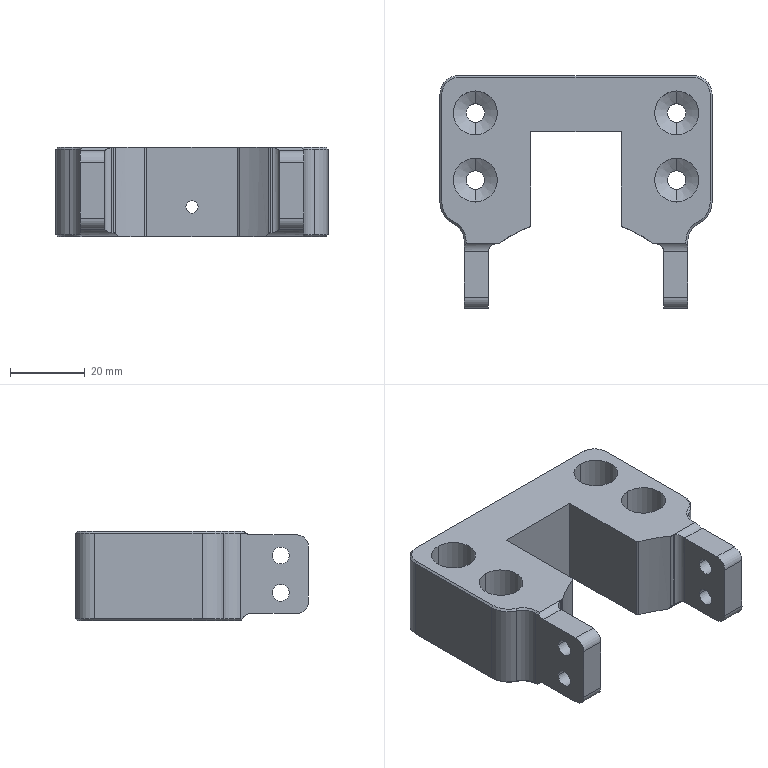NC program | NX | posted with a generic post | part box 73 x 62.4 x 24 mm
Lines 274 to 2248 of 2496, first 1642 of 1967 lines:
(ZLEVEL_PROFILE_COPY_1_COPY_1_COPY_1_1_COPY_1_COPY_1 , TOOL : D6R0.5)
N528 T05 M6
N530 G54
N532 G17 G0 G90 X30.873 Y-17.211 S8000 M3
N534 G43 Z30. H5
N536 Z1.406
N538 G94 G1 Z-0.094 F800.
N540 X30.42 Y-16.42
N542 G3 X29.901 Y-16.118 R0.6
N544 G1 X29.209 Y-16.115 F3000.
N546 X19.247 Y-16.117
N548 X19.161 Y-16.114
N550 X19.208 Y-16.149 Z-0.188
N552 X30. Y-16.15
N554 X30.098 Y-16.185 Z-0.281
N556 G3 X19.257 Y-16.185 R4880.801
N558 G1 X19.321 Y-16.22 Z-0.374
N560 X19.857 Y-16.214
N562 X29.549
N564 G3 X30.197 Y-16.223 R7.975
N566 G1 X30.275 Y-16.261 Z-0.467
N568 G2 X29.659 Y-16.251 R7.81
N570 G1 X19.921
N572 X19.385 Y-16.256
N574 X19.448 Y-16.295 Z-0.558
N576 X19.934 Y-16.297
N578 X19.991 Y-16.291
N580 X29.77
N582 G3 X30.338 Y-16.302 R5.245
N584 G1 X30.4 Y-16.348 Z-0.648
N586 X29.896 Y-16.338
N588 X29.877 Y-16.335
N590 X20.068
N592 G2 X19.51 Y-16.34 R3.857
N594 G1 X19.571 Y-16.389 Z-0.736
N596 G3 X20.149 Y-16.383 R13.947
N598 G1 X29.983
N600 G3 X30.461 Y-16.4 R3.808
N602 G1 X30.487 Y-16.458 Z-0.821
N604 X29.896 Y-16.445
N606 X29.817 Y-16.434
N608 X20.236
N610 X19.647 Y-16.443
N612 X19.733 Y-16.499 Z-0.904
N614 X20.331 Y-16.488
N616 X29.8
N618 X29.896 Y-16.506
N620 X30.489 Y-16.522
N622 X30.49 Y-16.551 Z-0.945
N624 X30.492 Y-16.584 Z-0.985
N626 X29.896 Y-16.565
N628 X29.784 Y-16.545
N630 X20.428
N632 X19.934 Y-16.558
N634 X19.817 Y-16.556
N636 X19.899 Y-16.612 Z-1.064
N638 X19.934 Y-16.613
N640 X20.526 Y-16.606
N642 X29.754
N644 X29.896 Y-16.63
N646 X30.494 Y-16.654
N648 X30.495 Y-16.692 Z-1.102
N650 X30.496 Y-16.725 Z-1.14
N652 G2 X29.734 Y-16.669 R3.451
N654 G1 X20.645
N656 X19.988 Y-16.673
N658 X20.082 Y-16.735 Z-1.213
N660 X20.835
N662 X29.714
N664 G3 X30.497 Y-16.798 R3.947
N666 G1 X30.498 Y-16.828 Z-1.248
N668 Y-16.876 Z-1.283
N670 G2 X29.705 Y-16.804 R3.354
N672 G1 X21.908
N674 X21.651 Y-16.809
N676 X20.277 Y-16.801
N678 X20.18 Y-16.798
N680 X20.283 Y-16.863 Z-1.35
N682 X20.621 Y-16.87
N684 X21.995 Y-16.885
N686 X22.199 Y-16.874
N688 X29.678
N690 X29.709 Y-16.895
N692 X29.896 Y-16.924
N694 X30.499 Y-16.951
N696 Y-16.985 Z-1.382
N698 Y-17.025 Z-1.414
N700 X29.896 Y-16.998
N702 X29.698 Y-16.97
N704 X29.666 Y-16.948
N706 X22.4
N708 X22.339 Y-16.952
N710 G2 X20.432 Y-16.927 R31.135
N712 G1 X20.573 Y-16.992 Z-1.475
N714 G3 X22.549 Y-17.028 R29.571
N716 G1 X22.56 Y-17.023
N718 X29.673
N720 G3 X30.499 Y-17.095 R3.382
N722 G1 Y-17.132 Z-1.504
N724 X30.5 Y-17.184 Z-1.533
N726 G2 X29.662 Y-17.101 R3.457
N728 G1 X22.131
N730 G2 X20.793 Y-17.058 R20.951
N732 G1 X20.955 Y-17.073 Z-1.54
N734 X21.118 Y-17.084 Z-1.548
N736 X21.28 Y-17.098 Z-1.556
N738 X21.443 Y-17.121 Z-1.564
N740 X21.605 Y-17.144 Z-1.572
N742 X21.767 Y-17.167 Z-1.579
N744 X21.929 Y-17.184 Z-1.587
N746 X22.682 Y-17.194
N748 X22.816 Y-17.18
N750 X29.622
N752 G3 X30.5 Y-17.272 R3.159
N754 G1 Y-17.313 Z-1.613
N756 Y-17.355 Z-1.638
N758 G2 X29.601 Y-17.26 R3.103
N760 G1 X22.919
N762 G2 X22.147 Y-17.271 R20.028
N764 G1 X22.224 Y-17.311 Z-1.662
N766 X22.301 Y-17.354 Z-1.686
N768 X23.01 Y-17.342
N770 X29.606
N772 G3 X30.5 Y-17.432 R3.176
N774 G1 Y-17.477 Z-1.707
N776 Y-17.53 Z-1.729
N778 X29.67 Y-17.451
N780 X29.584 Y-17.425
N782 X23.09
N784 X22.424 Y-17.436
N786 X22.522 Y-17.526 Z-1.77
N788 X23.162 Y-17.508
N790 X29.55
N792 G3 X30.5 Y-17.628 R3.156
N794 G1 Y-17.675 Z-1.788
N796 Y-17.717 Z-1.806
N798 G2 X29.522 Y-17.591 R3.218
N800 G1 X23.233
N802 X22.608 Y-17.615
N804 X22.685 Y-17.696 Z-1.839
N806 X23.288 Y-17.673
N808 X29.538
N810 G3 X30.5 Y-17.8 R3.249
N812 G1 Y-17.848 Z-1.853
N814 Y-17.907 Z-1.868
N816 X29.533 Y-17.754
N818 X23.33
N820 X22.749 Y-17.774
N822 X22.803 Y-17.853 Z-1.893
N824 X23.369 Y-17.833
N826 X29.468
N828 X29.553 Y-17.877
N830 X30.5 Y-18.004
N832 Y-18.046 Z-1.904
N834 Y-18.086 Z-1.915
N836 X29.514 Y-17.948
N838 X29.448 Y-17.91
N840 X23.398
N842 X22.848 Y-17.927
N844 X22.887 Y-17.999 Z-1.934
N846 X23.369 Y-18.011
N848 X23.425 Y-17.983
N850 X29.457
N852 X29.524 Y-18.021
N854 X30.5 Y-18.165
N856 Y-18.193 Z-1.942
N858 Y-18.257 Z-1.95
N860 X29.498 Y-18.058
N862 X23.448
N864 X23.369 Y-18.082
N866 X22.92 Y-18.079
N868 X22.947 Y-18.15 Z-1.963
N870 X23.026 Y-18.155
N872 X23.409 Y-18.138
N874 X23.466 Y-18.129
N876 X29.538
N878 G3 X30.5 Y-18.333 R2.976
N880 G1 Y-18.335 Z-1.968
N882 Y-18.393 Z-1.974
N884 G2 X29.547 Y-18.195 R2.825
N886 G1 X23.479
N888 X22.964 Y-18.256
N890 X22.976 Y-18.334 Z-1.981
N892 X23.026 Y-18.336
N894 X23.487 Y-18.252
N896 X29.561
N898 G3 X30.5 Y-18.436 R2.496
N900 G1 Z-1.984
N902 Y-18.465 Z-1.986
N904 G2 X29.615 Y-18.296 R1.899
N906 G1 X23.492
N908 X23.026 Y-18.386
N910 X22.984 Y-18.384
N912 G3 X22.454 Y-18.665 R0.6
N914 G1 X21.964 Y-19.446
N916 Z-0.486
N918 G0 Z30.
N920 X24.134 Y-19.644
N922 Z-0.5
N924 G1 Z-2. F800.
N926 X23.607 Y-18.622
N928 G2 X23.007 Y-18.595 R0.6
N930 G1 X23.026 Y-18.606 F3000.
N932 X23.034 Y-18.513
N934 G3 X23.5 Y-18.444 R0.591
N936 G1 X29.768
N938 X29.812 Y-18.454
N940 X30.511 Y-18.568
N942 G2 X30.976 Y-18.947 R0.6
N944 G1 X31.255 Y-19.681
N946 Z-0.5
N948 G0 Z30.
N950 X-18.139 Y-17.192
N952 Z1.406
N954 G1 Z-0.094 F800.
N956 X-18.632 Y-16.397
N958 G3 X-19.161 Y-16.113 R0.6
N960 G1 X-19.247 Y-16.116 F3000.
N962 X-29.209
N964 X-29.904 Y-16.122
N966 X-30.003 Y-16.153 Z-0.188
N968 X-29.553 Y-16.151
N970 X-19.207 Y-16.148
N972 X-19.256 Y-16.184 Z-0.281
N974 X-29.553 Y-16.185
N976 X-30.102 Y-16.188
N978 X-30.2 Y-16.226 Z-0.374
N980 G3 X-29.549 Y-16.214 R9.826
N982 G1 X-19.857
N984 X-19.321 Y-16.22
N986 X-19.385 Y-16.257 Z-0.467
N988 X-19.921 Y-16.251
N990 X-29.553
N992 X-29.588 Y-16.253
N994 X-30.24 Y-16.265
N996 X-30.279 Y-16.264
N998 X-30.344 Y-16.303 Z-0.558
N1000 G3 X-29.77 Y-16.291 R5.171
N1002 G1 X-19.991
N1004 X-19.934 Y-16.298
N1006 X-19.448
N1008 X-19.51 Y-16.344 Z-0.648
N1010 G2 X-20.068 Y-16.335 R3.757
N1012 G1 X-29.553
N1014 X-30.408 Y-16.35
N1016 X-30.47 Y-16.404 Z-0.736
N1018 X-29.983 Y-16.383
N1020 X-20.149
N1022 G3 X-19.57 Y-16.39 R6.048
N1024 G1 X-19.646 Y-16.442 Z-0.821
N1026 X-20.236 Y-16.434
N1028 X-29.882
N1030 X-29.893 Y-16.438
N1032 X-30.488 Y-16.465
N1034 X-30.49 Y-16.498 Z-0.863
N1036 X-30.491 Y-16.528 Z-0.904
N1038 G3 X-29.856 Y-16.488 R4.144
N1040 G1 X-20.331
N1042 X-19.733 Y-16.499
N1044 X-19.817 Y-16.556 Z-0.985
N1046 X-19.934 Y-16.559
N1048 X-20.428 Y-16.545
N1050 X-29.832
N1052 G2 X-30.493 Y-16.589 R4.026
N1054 G1 X-30.494 Y-16.628 Z-1.025
N1056 X-30.495 Y-16.66 Z-1.064
N1058 X-29.896 Y-16.629
N1060 X-29.766 Y-16.606
N1062 X-20.526
N1064 X-19.934 Y-16.615
N1066 X-19.899 Y-16.613
N1068 X-19.988 Y-16.674 Z-1.14
N1070 X-20.645 Y-16.669
N1072 X-29.738
N1074 G2 X-30.497 Y-16.728 R3.659
N1076 G1 Y-16.764 Z-1.176
N1078 X-30.498 Y-16.799 Z-1.213
N1080 G3 X-29.733 Y-16.735 R3.594
N1082 G1 X-20.835
N1084 X-20.081 Y-16.736
N1086 X-20.176 Y-16.801 Z-1.283
N1088 X-21.651 Y-16.805
N1090 X-21.908 Y-16.804
N1092 X-29.722
N1094 G2 X-30.498 Y-16.873 R2.822
N1096 G1 X-30.499 Y-16.906 Z-1.316
N1098 Y-16.944 Z-1.35
N1100 G3 X-29.677 Y-16.874 R3.006
N1102 G1 X-22.199
N1104 X-21.995 Y-16.877
N1106 X-20.621 Y-16.864
N1108 X-20.281
N1110 X-20.368 Y-16.894 Z-1.382
N1112 X-20.454 Y-16.93 Z-1.414
N1114 X-22.4 Y-16.948
N1116 X-29.662
N1118 G2 X-30.499 Y-17.021 R2.714
N1120 G1 Y-17.061 Z-1.444
N1122 X-30.5 Y-17.095 Z-1.475
N1124 G3 X-29.677 Y-17.023 R3.287
N1126 G1 X-22.56
N1128 X-22.547 Y-17.028
N1130 X-20.619 Y-17.009
N1132 X-20.77 Y-17.035 Z-1.489
N1134 X-20.921 Y-17.059 Z-1.504
N1136 X-21.073 Y-17.079 Z-1.518
N1138 X-21.224 Y-17.098 Z-1.533
N1140 X-22.698 Y-17.101
N1142 X-29.662
N1144 G2 X-30.5 Y-17.184 R3.452
N1146 G1 Y-17.225 Z-1.56
N1148 Y-17.273 Z-1.587
N1150 G3 X-29.622 Y-17.18 R3.151
N1152 G1 X-22.816
N1154 X-22.682 Y-17.193
N1156 X-21.855 Y-17.179
N1158 X-21.992 Y-17.223 Z-1.613
N1160 X-22.129 Y-17.268 Z-1.638
N1162 G2 X-22.919 Y-17.26 R18.795
N1164 G1 X-29.601
N1166 G2 X-30.5 Y-17.355 R3.09
N1168 G1 Y-17.395 Z-1.662
N1170 Y-17.432 Z-1.686
N1172 G3 X-29.606 Y-17.342 R3.157
N1174 G1 X-23.01
N1176 X-22.299 Y-17.353
N1178 X-22.426 Y-17.435 Z-1.729
N1180 X-23.026 Y-17.43
N1182 X-23.09 Y-17.425
N1184 X-29.585
N1186 X-29.668 Y-17.451
N1188 X-30.5 Y-17.529
N1190 Y-17.579 Z-1.749
N1192 Y-17.626 Z-1.77
N1194 G3 X-29.54 Y-17.508 R3.199
N1196 G1 X-23.162
N1198 X-22.523 Y-17.527
N1200 X-22.61 Y-17.616 Z-1.806
N1202 X-23.222 Y-17.591
N1204 X-29.523
N1206 G2 X-30.5 Y-17.714 R3.105
N1208 G1 Y-17.756 Z-1.822
N1210 Y-17.795 Z-1.839
N1212 G3 X-29.528 Y-17.673 R3.208
N1214 G1 X-23.277
N1216 X-22.688 Y-17.699
N1218 X-22.753 Y-17.778 Z-1.868
N1220 X-23.323 Y-17.754
N1222 X-29.522
N1224 G2 X-30.5 Y-17.894 R2.967
N1226 G1 Y-17.936 Z-1.88
N1228 Y-17.985 Z-1.893
N1230 X-29.553 Y-17.878
N1232 X-29.47 Y-17.833
N1234 X-23.365
N1236 X-22.806 Y-17.857
N1238 X-22.85 Y-17.928 Z-1.915
N1240 X-23.398 Y-17.91
N1242 X-29.448
N1244 X-29.553 Y-17.964
N1246 X-30.5 Y-18.062
N1248 Y-18.095 Z-1.924
N1250 Y-18.127 Z-1.934
N1252 X-29.553 Y-18.037
N1254 X-29.457 Y-17.983
N1256 X-23.425
N1258 X-23.369 Y-18.01
N1260 X-22.888 Y-18.
N1262 X-22.921 Y-18.078 Z-1.95
N1264 X-23.369 Y-18.081
N1266 X-23.448 Y-18.058
N1268 X-29.496
N1270 G2 X-30.499 Y-18.208 R2.092
N1272 G1 Y-18.217 Z-1.956
N1274 X-30.497 Y-18.278 Z-1.963
N1276 G3 X-29.525 Y-18.129 R1.386
N1278 G1 X-23.466
N1280 X-23.417 Y-18.138
N1282 X-23.026 Y-18.154
N1284 X-22.947 Y-18.149
N1286 X-22.952 Y-18.183 Z-1.968
N1288 X-22.964 Y-18.255 Z-1.974
N1290 X-23.479 Y-18.195
N1292 X-29.538
N1294 G2 X-30.496 Y-18.34 R1.226
N1296 G1 X-30.497 Y-18.355 Z-1.978
N1298 X-30.499 Y-18.401 Z-1.981
N1300 G3 X-29.553 Y-18.252 R1.279
N1302 G1 X-23.487
N1304 X-23.026 Y-18.336
N1306 X-22.976 Y-18.334
N1308 X-22.984 Y-18.384 Z-1.986
N1310 X-23.026 Y-18.386
N1312 X-23.492 Y-18.296
N1314 X-29.576
N1316 G2 X-30.499 Y-18.44 R1.314
N1318 G1 Y-18.5 Z-1.993
N1320 Y-18.548 Z-2.
N1322 G3 X-29.605 Y-18.444 R2.193
N1324 G1 X-23.5
N1326 G3 X-22.994 Y-18.518 R0.808
N1328 G1 Z-0.5
N1330 G0 Z30.
(ZLEVEL_PROFILE_COPY_1_COPY_1_COPY_1_1_COPY_1_COPY_COPY , TOOL : D6R0.5)
N1332 X-21.887 Y-31.829
N1334 Z-0.508
N1336 G1 Z-2.008 F800.
N1338 X-22.714 Y-30.914
N1340 G3 X-23. Y-30.822 R0.3
N1342 G1 X-23.5 Y-30.93 F3000.
N1344 X-30.
N1346 X-30.5 Y-30.822
N1348 Y-30.937 Z-2.012
N1350 Y-30.954 Z-2.017
N1352 X-30. Y-31.045
N1354 X-23.5
N1356 X-23. Y-30.954
N1358 Y-31.044 Z-2.023
N1360 Y-31.092 Z-2.029
N1362 X-23.5 Y-31.152
N1364 X-30.
N1366 X-30.456 Y-31.106
N1368 X-30.497 Y-31.102
N1370 X-30.583 Y-31.138 Z-2.037
N1372 X-30.665 Y-31.159 Z-2.044
N1374 X-30.623 Y-31.179
N1376 X-30. Y-31.256
N1378 X-23.5
N1380 X-23. Y-31.18
N1382 Y-31.257 Z-2.053
N1384 Y-31.284 Z-2.062
N1386 X-23.5 Y-31.357
N1388 X-30.
N1390 X-30.507 Y-31.307
N1392 X-30.624 Y-31.281
N1394 X-30.563 Y-31.346 Z-2.072
N1396 X-30.5 Y-31.408 Z-2.083
N1398 X-30.438 Y-31.416
N1400 X-30. Y-31.456
N1402 X-23.5
N1404 X-23.063 Y-31.416
N1406 X-23. Y-31.403
N1408 X-22.988 Y-31.456 Z-2.094
N1410 X-22.979 Y-31.494 Z-2.106
N1412 X-23.5 Y-31.555
N1414 X-30.
N1416 X-30.38 Y-31.51
N1418 Y-31.573 Z-2.118
N1420 Y-31.605 Z-2.131
N1422 X-30. Y-31.648
N1424 X-23.5
N1426 X-22.953 Y-31.588
N1428 X-22.928 Y-31.634 Z-2.146
N1430 X-22.947 Y-31.641
N1432 X-23.5 Y-31.701
N1434 X-30.
N1436 X-30.553 Y-31.641
N1438 X-30.573 Y-31.634
N1440 X-30.635 Y-31.705 Z-2.174
N1442 X-30.553 Y-31.731
N1444 X-30. Y-31.791
N1446 X-23.5
N1448 X-22.947 Y-31.731
N1450 X-22.869 Y-31.707
N1452 X-22.949 Y-31.828 Z-2.207
N1454 X-23.5 Y-31.886
N1456 X-30.
N1458 X-30.551 Y-31.828
N1460 X-30.534 Y-31.917 Z-2.243
N1462 X-30. Y-31.98
N1464 X-23.5
N1466 X-22.966 Y-31.917
N1468 X-22.984 Y-32.014 Z-2.281
N1470 X-23.5 Y-32.073
N1472 X-30.
N1474 X-30.516 Y-32.014
N1476 X-30.506 Y-32.116 Z-2.321
N1478 X-30.434 Y-32.128
N1480 X-30. Y-32.165
N1482 X-23.5
N1484 X-23.066 Y-32.128
N1486 X-22.994 Y-32.116
N1488 X-22.888 Y-32.132 Z-2.339
N1490 X-22.784 Y-32.143 Z-2.357
N1492 G2 X-23.5 Y-32.239 R3.29
N1494 G1 X-30.
N1496 X-30.525 Y-32.186
N1498 X-30.553 Y-32.181
N1500 Y-32.226 Z-2.379
N1502 Y-32.271 Z-2.401
N1504 X-30.456 Y-32.289
N1506 X-30. Y-32.327
N1508 X-23.5
N1510 G3 X-22.774 Y-32.235 R5.494
N1512 G1 X-22.886 Y-32.301 Z-2.425
N1514 X-22.997 Y-32.368 Z-2.449
N1516 X-23.033 Y-32.375
N1518 X-23.5 Y-32.415
N1520 X-30.
N1522 X-30.467 Y-32.375
N1524 X-30.503 Y-32.368
N1526 X-30.501 Y-32.413 Z-2.474
N1528 X-30.5 Y-32.455 Z-2.499
N1530 X-30. Y-32.502
N1532 X-23.5
N1534 X-23.12 Y-32.474
N1536 X-23.042 Y-32.462
N1538 X-23.038 Y-32.505 Z-2.526
N1540 X-23.034 Y-32.541 Z-2.552
N1542 X-23.12 Y-32.558
N1544 X-23.5 Y-32.587
N1546 X-30.
N1548 X-30.5 Y-32.534
N1550 Y-32.583 Z-2.58
N1552 Y-32.616 Z-2.607
N1554 G3 X-30. Y-32.67 R2.266
N1556 G1 X-23.5
N1558 X-23.12 Y-32.643
N1560 X-23.034 Y-32.623
N1562 Y-32.671 Z-2.636
N1564 Y-32.706 Z-2.665
N1566 X-23.12 Y-32.723
N1568 X-23.5 Y-32.752
N1570 X-30.
N1572 X-30.5 Y-32.699
N1574 Y-32.747 Z-2.695
N1576 Y-32.786 Z-2.724
N1578 X-30. Y-32.832
N1580 X-23.5
N1582 X-22.993 Y-32.784
N1584 X-22.997 Y-32.827 Z-2.756
N1586 X-23. Y-32.861 Z-2.787
N1588 X-23.5 Y-32.911
N1590 X-30.
N1592 X-30.5 Y-32.861
N1594 Y-32.905 Z-2.819
N1596 Y-32.937 Z-2.851
N1598 G3 X-30. Y-32.987 R3.643
N1600 G1 X-23.5
N1602 G3 X-23. Y-32.937 R11.191
N1604 G1 Y-32.98 Z-2.884
N1606 Y-33.012 Z-2.917
N1608 X-23.5 Y-33.062
N1610 X-30.
N1612 X-30.5 Y-33.012
N1614 Y-33.054 Z-2.952
N1616 Y-33.087 Z-2.986
N1618 G3 X-30. Y-33.135 R4.055
N1620 G1 X-23.5
N1622 G3 X-23. Y-33.087 R16.285
N1624 G1 Y-33.127 Z-3.021
N1626 Y-33.158 Z-3.056
N1628 G2 X-23.5 Y-33.206 R8.587
N1630 G1 X-30.
N1632 G2 X-30.5 Y-33.158 R5.074
N1634 G1 Y-33.197 Z-3.093
N1636 Y-33.225 Z-3.129
N1638 G3 X-30. Y-33.275 R5.013
N1640 G1 X-23.5
N1642 G3 X-23. Y-33.225 R2.863
N1644 G1 X-22.999 Y-33.263 Z-3.166
N1646 Y-33.293 Z-3.204
N1648 G2 X-23.5 Y-33.341 R2.836
N1650 G1 X-30.
N1652 G2 X-30.501 Y-33.293 R4.426
N1654 G1 Y-33.329 Z-3.242
N1656 Y-33.357 Z-3.28
N1658 G3 X-30. Y-33.406 R4.48
N1660 G1 X-23.5
N1662 G3 X-22.999 Y-33.357 R19.399
N1664 G1 X-23. Y-33.393 Z-3.319
N1666 Y-33.42 Z-3.358
N1668 G2 X-23.5 Y-33.468 R2.805
N1670 G1 X-30.
N1672 G2 X-30.5 Y-33.42 R4.824
N1674 G1 Y-33.455 Z-3.398
N1676 Y-33.484 Z-3.438
N1678 G3 X-30. Y-33.528 R3.789
N1680 G1 X-23.5
N1682 G3 X-23. Y-33.484 R3.788
N1684 G1 Y-33.514 Z-3.479
N1686 Y-33.538 Z-3.52
N1688 G2 X-23.5 Y-33.586 R3.559
N1690 G1 X-30.
N1692 G2 X-30.5 Y-33.538 R4.017
N1694 G1 X-30.501 Y-33.57 Z-3.561
N1696 Y-33.592 Z-3.603
N1698 G3 X-30. Y-33.641 R3.739
N1700 G1 X-23.5
N1702 G3 X-22.999 Y-33.592 R2.773
N1704 G1 Y-33.624 Z-3.645
N1706 X-22.998 Y-33.647 Z-3.688
N1708 G2 X-23.5 Y-33.694 R3.345
N1710 G1 X-30.
N1712 G2 X-30.502 Y-33.647 R5.322
N1714 G1 X-30.501 Y-33.676 Z-3.731
N1716 Y-33.696 Z-3.774
N1718 G3 X-30. Y-33.745 R4.043
N1720 G1 X-23.5
N1722 G3 X-22.999 Y-33.696 R3.86
N1724 G1 Y-33.725 Z-3.818
N1726 Y-33.743 Z-3.862
N1728 G2 X-23.5 Y-33.793 R3.817
N1730 G1 X-30.
N1732 G2 X-30.501 Y-33.743 R3.826
N1734 G1 X-30.5 Y-33.772 Z-3.906
N1736 Y-33.791 Z-3.951
N1738 G3 X-30. Y-33.839 R3.505
N1740 G1 X-23.5
N1742 G3 X-23. Y-33.791 R3.49
N1744 G1 Y-33.817 Z-3.996
N1746 Y-33.837 Z-4.041
N1748 G2 X-23.5 Y-33.881 R3.205
N1750 G1 X-30.
N1752 G2 X-30.5 Y-33.837 R4.155
N1754 G1 X-30.501 Y-33.859 Z-4.087
N1756 X-30.502 Y-33.874 Z-4.133
N1758 G3 X-30. Y-33.922 R3.739
N1760 G1 X-23.5
N1762 G3 X-22.998 Y-33.874 R3.712
N1764 G1 Y-33.897 Z-4.179
N1766 X-22.997 Y-33.911 Z-4.225
N1768 G2 X-23.5 Y-33.96 R3.842
N1770 G1 X-30.
N1772 G2 X-30.503 Y-33.911 R3.883
N1774 G1 Y-33.933 Z-4.272
N1776 X-30.504 Y-33.949 Z-4.319
N1778 G3 X-30. Y-33.995 R4.036
N1780 G1 X-23.5
N1782 G3 X-22.996 Y-33.948 R3.978
N1784 G1 Y-33.968 Z-4.366
N1786 Y-33.985 Z-4.414
N1788 G2 X-23.5 Y-34.027 R4.104
N1790 G1 X-30.
N1792 G2 X-30.504 Y-33.986 R5.724
N1794 G1 Y-34.001 Z-4.461
N1796 Y-34.018 Z-4.509
N1798 G3 X-30. Y-34.057 R5.944
N1800 G1 X-23.5
N1802 G3 X-22.996 Y-34.016 R5.138
N1804 G1 X-22.995 Y-34.026 Z-4.557
N1806 Y-34.042 Z-4.605
N1808 G2 X-23.5 Y-34.084 R3.614
N1810 G1 X-30.
N1812 G2 X-30.504 Y-34.045 R6.41
N1814 G1 Y-34.055 Z-4.654
N1816 Y-34.072 Z-4.702
N1818 G3 X-30. Y-34.108 R6.488
N1820 G1 X-23.5
N1822 G3 X-22.996 Y-34.067 R3.742
N1824 G1 Y-34.076 Z-4.751
N1826 Y-34.092 Z-4.8
N1828 G2 X-23.5 Y-34.129 R4.148
N1830 G1 X-30.
N1832 X-30.503 Y-34.099
N1834 X-30.502 Y-34.106 Z-4.849
N1836 Y-34.125 Z-4.898
N1838 X-30. Y-34.148
N1840 X-23.5
N1842 X-22.998 Y-34.115
N1844 Y-34.122 Z-4.948
N1846 X-22.999 Y-34.136 Z-4.997
N1848 X-23.5 Y-34.164
N1850 X-30.
N1852 X-30.501 Y-34.143
N1854 Y-34.15 Z-5.047
N1856 X-30.5 Y-34.159 Z-5.096
N1858 X-30. Y-34.177
N1860 X-23.5
N1862 X-23. Y-34.153
N1864 Y-34.162 Z-5.146
N1866 Y-34.17 Z-5.196
N1868 X-23.5 Y-34.187
N1870 X-30.
N1872 X-30.492 Y-34.174
N1874 X-30.465 Y-34.181 Z-5.272
N1876 X-30. Y-34.193
N1878 X-23.5
N1880 X-23.026 Y-34.179
N1882 X-23.054 Y-34.188 Z-5.348
N1884 X-23.5 Y-34.197
N1886 X-30.
N1888 X-30.438 Y-34.188
N1890 X-30.411 Y-34.195 Z-5.424
N1892 X-29.861 Y-34.197
N1894 X-23.639
N1896 X-23.081 Y-34.195
N1898 X-23.11 Y-34.197 Z-5.5
N1900 X-29.861 Y-34.198
N1902 X-30.384 Y-34.197
N1904 G3 X-30.904 Y-34.497 R0.6
N1906 G1 X-31.374 Y-35.308
N1908 Z-4.
N1910 G0 Z30.
N1912 X31.613 Y-31.829
N1914 Z-0.508
N1916 G1 Z-2.008 F800.
N1918 X30.786 Y-30.914
N1920 G3 X30.5 Y-30.822 R0.3
N1922 G1 X30. Y-30.93 F3000.
N1924 X23.5
N1926 X23. Y-30.822
N1928 Y-30.937 Z-2.012
N1930 Y-30.954 Z-2.017
N1932 X23.5 Y-31.045
N1934 X30.
N1936 X30.5 Y-30.954
N1938 Y-31.044 Z-2.023
N1940 Y-31.092 Z-2.029
N1942 X30. Y-31.152
N1944 X23.5
N1946 X23.044 Y-31.106
N1948 X23.003 Y-31.102
N1950 X22.917 Y-31.138 Z-2.037
N1952 X22.835 Y-31.159 Z-2.044
N1954 X22.877 Y-31.179
N1956 X23.5 Y-31.256
N1958 X30.
N1960 X30.5 Y-31.18
N1962 Y-31.257 Z-2.053
N1964 Y-31.284 Z-2.062
N1966 X30. Y-31.357
N1968 X23.5
N1970 X22.993 Y-31.307
N1972 X22.876 Y-31.281
N1974 X22.937 Y-31.346 Z-2.072
N1976 X23. Y-31.408 Z-2.083
N1978 X23.062 Y-31.416
N1980 X23.5 Y-31.456
N1982 X30.
N1984 X30.437 Y-31.416
N1986 X30.5 Y-31.403
N1988 X30.512 Y-31.456 Z-2.094
N1990 X30.521 Y-31.494 Z-2.106
N1992 X30. Y-31.555
N1994 X23.5
N1996 X23.12 Y-31.51
N1998 Y-31.573 Z-2.118
N2000 Y-31.605 Z-2.131
N2002 X23.5 Y-31.648
N2004 X30.
N2006 X30.547 Y-31.588
N2008 X30.572 Y-31.634 Z-2.146
N2010 X30.553 Y-31.641
N2012 X30. Y-31.701
N2014 X23.5
N2016 X22.947 Y-31.641
N2018 X22.927 Y-31.634
N2020 X22.865 Y-31.705 Z-2.174
N2022 X22.947 Y-31.731
N2024 X23.5 Y-31.791
N2026 X30.
N2028 X30.553 Y-31.731
N2030 X30.631 Y-31.707
N2032 X30.551 Y-31.828 Z-2.207
N2034 X30. Y-31.886
N2036 X23.5
N2038 X22.949 Y-31.828
N2040 X22.966 Y-31.917 Z-2.243
N2042 X23.5 Y-31.98
N2044 X30.
N2046 X30.534 Y-31.917
N2048 X30.516 Y-32.014 Z-2.281
N2050 X30. Y-32.073
N2052 X23.5
N2054 X22.984 Y-32.014
N2056 X22.994 Y-32.116 Z-2.321
N2058 X23.066 Y-32.128
N2060 X23.5 Y-32.165
N2062 X30.
N2064 X30.434 Y-32.128
N2066 X30.506 Y-32.116
N2068 X30.612 Y-32.132 Z-2.339
N2070 X30.716 Y-32.143 Z-2.357
N2072 G2 X30. Y-32.239 R3.29
N2074 G1 X23.5
N2076 X22.975 Y-32.186
N2078 X22.947 Y-32.181
N2080 Y-32.226 Z-2.379
N2082 Y-32.271 Z-2.401
N2084 X23.044 Y-32.289
N2086 X23.5 Y-32.327
N2088 X30.
N2090 G3 X30.726 Y-32.235 R5.494
N2092 G1 X30.614 Y-32.301 Z-2.425
N2094 X30.503 Y-32.368 Z-2.449
N2096 X30.467 Y-32.375
N2098 X30. Y-32.415
N2100 X23.5
N2102 X23.033 Y-32.375
N2104 X22.997 Y-32.368
N2106 X22.999 Y-32.413 Z-2.474
N2108 X23. Y-32.455 Z-2.499
N2110 X23.5 Y-32.502
N2112 X30.
N2114 X30.38 Y-32.474
N2116 X30.458 Y-32.462
N2118 X30.462 Y-32.505 Z-2.526
N2120 X30.466 Y-32.541 Z-2.552
N2122 X30.38 Y-32.558
N2124 X30. Y-32.587
N2126 X23.5
N2128 X23. Y-32.534
N2130 Y-32.583 Z-2.58
N2132 Y-32.616 Z-2.607
N2134 G3 X23.5 Y-32.67 R2.266
N2136 G1 X30.
N2138 X30.38 Y-32.643
N2140 X30.466 Y-32.623
N2142 Y-32.671 Z-2.636
N2144 Y-32.706 Z-2.665
N2146 X30.38 Y-32.723
N2148 X30. Y-32.752
N2150 X23.5
N2152 X23. Y-32.699
N2154 Y-32.747 Z-2.695
N2156 Y-32.786 Z-2.724
N2158 X23.5 Y-32.832
N2160 X30.
N2162 X30.507 Y-32.784
N2164 X30.503 Y-32.827 Z-2.756
N2166 X30.5 Y-32.861 Z-2.787
N2168 X30. Y-32.911
N2170 X23.5
N2172 X23. Y-32.861
N2174 Y-32.905 Z-2.819
N2176 Y-32.937 Z-2.851
N2178 G3 X23.5 Y-32.987 R3.643
N2180 G1 X30.
N2182 G3 X30.5 Y-32.937 R11.191
N2184 G1 Y-32.98 Z-2.884
N2186 Y-33.012 Z-2.917
N2188 X30. Y-33.062
N2190 X23.5
N2192 X23. Y-33.012
N2194 Y-33.054 Z-2.952
N2196 Y-33.087 Z-2.986
N2198 G3 X23.5 Y-33.135 R4.055
N2200 G1 X30.
N2202 G3 X30.5 Y-33.087 R16.285
N2204 G1 Y-33.127 Z-3.021
N2206 Y-33.158 Z-3.056
N2208 G2 X30. Y-33.206 R8.587
N2210 G1 X23.5
N2212 G2 X23. Y-33.158 R5.074
N2214 G1 Y-33.197 Z-3.093
N2216 Y-33.225 Z-3.129
N2218 G3 X23.5 Y-33.275 R5.013
N2220 G1 X30.
N2222 G3 X30.5 Y-33.225 R2.863
N2224 G1 X30.501 Y-33.263 Z-3.166
N2226 Y-33.293 Z-3.204
N2228 G2 X30. Y-33.341 R2.836
N2230 G1 X23.5
N2232 G2 X22.999 Y-33.293 R4.426
N2234 G1 Y-33.329 Z-3.242
N2236 Y-33.357 Z-3.28
N2238 G3 X23.5 Y-33.406 R4.48
N2240 G1 X30.
N2242 G3 X30.501 Y-33.357 R19.399
N2244 G1 X30.5 Y-33.393 Z-3.319
N2246 Y-33.42 Z-3.358
N2248 G2 X30. Y-33.468 R2.805
N2250 G1 X23.5
N2252 G2 X23. Y-33.42 R4.824
N2254 G1 Y-33.455 Z-3.398
N2256 Y-33.484 Z-3.438
N2258 G3 X23.5 Y-33.528 R3.789
N2260 G1 X30.
N2262 G3 X30.5 Y-33.484 R3.788
N2264 G1 Y-33.514 Z-3.479
N2266 Y-33.538 Z-3.52
N2268 G2 X30. Y-33.586 R3.559
N2270 G1 X23.5
N2272 G2 X23. Y-33.538 R4.017
N2274 G1 X22.999 Y-33.57 Z-3.561
N2276 Y-33.592 Z-3.603
N2278 G3 X23.5 Y-33.641 R3.739
N2280 G1 X30.
N2282 G3 X30.501 Y-33.592 R2.773
N2284 G1 Y-33.624 Z-3.645
N2286 X30.502 Y-33.647 Z-3.688
N2288 G2 X30. Y-33.694 R3.345
N2290 G1 X23.5
N2292 G2 X22.998 Y-33.647 R5.322
N2294 G1 X22.999 Y-33.676 Z-3.731
N2296 Y-33.696 Z-3.774
N2298 G3 X23.5 Y-33.745 R4.043
N2300 G1 X30.
N2302 G3 X30.501 Y-33.696 R3.86
N2304 G1 Y-33.725 Z-3.818
N2306 Y-33.743 Z-3.862
N2308 G2 X30. Y-33.793 R3.817
N2310 G1 X23.5
N2312 G2 X22.999 Y-33.743 R3.826
N2314 G1 X23. Y-33.772 Z-3.906
N2316 Y-33.791 Z-3.951
N2318 G3 X23.5 Y-33.839 R3.505
N2320 G1 X30.
N2322 G3 X30.5 Y-33.791 R3.49
N2324 G1 Y-33.817 Z-3.996
N2326 Y-33.837 Z-4.041
N2328 G2 X30. Y-33.881 R3.205
N2330 G1 X23.5
N2332 G2 X23. Y-33.837 R4.155
N2334 G1 X22.999 Y-33.859 Z-4.087
N2336 X22.998 Y-33.874 Z-4.133
N2338 G3 X23.5 Y-33.922 R3.739
N2340 G1 X30.
N2342 G3 X30.502 Y-33.874 R3.712
N2344 G1 Y-33.897 Z-4.179
N2346 X30.503 Y-33.911 Z-4.225
N2348 G2 X30. Y-33.96 R3.842
N2350 G1 X23.5
N2352 G2 X22.997 Y-33.911 R3.883
N2354 G1 Y-33.933 Z-4.272
N2356 X22.996 Y-33.949 Z-4.319
N2358 G3 X23.5 Y-33.995 R4.036
N2360 G1 X30.
N2362 G3 X30.504 Y-33.948 R3.978
N2364 G1 Y-33.968 Z-4.366
N2366 Y-33.985 Z-4.414
N2368 G2 X30. Y-34.027 R4.104
N2370 G1 X23.5
N2372 G2 X22.996 Y-33.986 R5.724
N2374 G1 Y-34.001 Z-4.461
N2376 Y-34.018 Z-4.509
N2378 G3 X23.5 Y-34.057 R5.944
N2380 G1 X30.
N2382 G3 X30.504 Y-34.016 R5.138
N2384 G1 X30.505 Y-34.026 Z-4.557
N2386 Y-34.042 Z-4.605
N2388 G2 X30. Y-34.084 R3.614
N2390 G1 X23.5
N2392 G2 X22.996 Y-34.045 R6.41
N2394 G1 Y-34.055 Z-4.654
N2396 Y-34.072 Z-4.702
N2398 G3 X23.5 Y-34.108 R6.488
N2400 G1 X30.
N2402 G3 X30.504 Y-34.067 R3.742
N2404 G1 Y-34.076 Z-4.751
N2406 Y-34.092 Z-4.8
N2408 G2 X30. Y-34.129 R4.148
N2410 G1 X23.5
N2412 X22.997 Y-34.099
N2414 X22.998 Y-34.106 Z-4.849
N2416 Y-34.125 Z-4.898
N2418 X23.5 Y-34.148
N2420 X30.
N2422 X30.502 Y-34.115
N2424 Y-34.122 Z-4.948
N2426 X30.501 Y-34.136 Z-4.997
N2428 X30. Y-34.164
N2430 X23.5
N2432 X22.999 Y-34.143
N2434 Y-34.15 Z-5.047
N2436 X23. Y-34.159 Z-5.096
N2438 X23.5 Y-34.177
N2440 X30.
N2442 X30.5 Y-34.153
N2444 Y-34.162 Z-5.146
N2446 Y-34.17 Z-5.196
N2448 X30. Y-34.187
N2450 X23.5
N2452 X23.008 Y-34.174
N2454 X23.035 Y-34.181 Z-5.272
N2456 X23.5 Y-34.193
N2458 X30.
N2460 X30.474 Y-34.179
N2462 X30.446 Y-34.188 Z-5.348
N2464 X30. Y-34.197
N2466 X23.5
N2468 X23.062 Y-34.188
N2470 X23.089 Y-34.195 Z-5.424
N2472 X23.639 Y-34.197
N2474 X29.861
N2476 X30.419 Y-34.195
N2478 X30.39 Y-34.197 Z-5.5
N2480 X23.639 Y-34.198
N2482 X23.116 Y-34.197
N2484 G3 X22.596 Y-34.497 R0.6
N2486 G1 X22.126 Y-35.308
N2488 Z-4.
N2490 G0 Z30.
(ZLEVEL_PROFILE_COPY_1_COPY_1_COPY_1_1_COPY_1_COPY_1_COPY , TOOL : D6R0.5)
N2492 G55
N2494 X30.873 Y-17.211
N2496 Z1.406
N2498 G1 Z-0.094 F800.
N2500 X30.42 Y-16.42
N2502 G3 X29.901 Y-16.118 R0.6
N2504 G1 X29.209 Y-16.115 F3000.
N2506 X19.247 Y-16.117
N2508 X19.161 Y-16.114
N2510 X19.208 Y-16.149 Z-0.188
N2512 X30. Y-16.15
N2514 X30.098 Y-16.185 Z-0.281
N2516 G3 X19.257 Y-16.185 R4880.801
N2518 G1 X19.321 Y-16.22 Z-0.374
N2520 X19.857 Y-16.214
N2522 X29.549
N2524 G3 X30.197 Y-16.223 R7.975
N2526 G1 X30.275 Y-16.261 Z-0.467
N2528 G2 X29.659 Y-16.251 R7.81
N2530 G1 X19.921
N2532 X19.385 Y-16.256
N2534 X19.448 Y-16.295 Z-0.558
N2536 X19.934 Y-16.297
N2538 X19.991 Y-16.291
N2540 X29.77
N2542 G3 X30.338 Y-16.302 R5.245
N2544 G1 X30.4 Y-16.348 Z-0.648
N2546 X29.896 Y-16.338
N2548 X29.877 Y-16.335
N2550 X20.068
N2552 G2 X19.51 Y-16.34 R3.857
N2554 G1 X19.571 Y-16.389 Z-0.736
N2556 G3 X20.149 Y-16.383 R13.947
N2558 G1 X29.983
N2560 G3 X30.461 Y-16.4 R3.808
N2562 G1 X30.487 Y-16.458 Z-0.821
N2564 X29.896 Y-16.445
N2566 X29.817 Y-16.434
N2568 X20.236
N2570 X19.647 Y-16.443
N2572 X19.733 Y-16.499 Z-0.904
N2574 X20.331 Y-16.488
N2576 X29.8
N2578 X29.896 Y-16.506
N2580 X30.489 Y-16.522
N2582 X30.49 Y-16.551 Z-0.945
N2584 X30.492 Y-16.584 Z-0.985
N2586 X29.896 Y-16.565
N2588 X29.784 Y-16.545
N2590 X20.428
N2592 X19.934 Y-16.558
N2594 X19.817 Y-16.556
N2596 X19.899 Y-16.612 Z-1.064
N2598 X19.934 Y-16.613
N2600 X20.526 Y-16.606
N2602 X29.754
N2604 X29.896 Y-16.63
N2606 X30.494 Y-16.654
N2608 X30.495 Y-16.692 Z-1.102
N2610 X30.496 Y-16.725 Z-1.14
N2612 G2 X29.734 Y-16.669 R3.451
N2614 G1 X20.645
N2616 X19.988 Y-16.673
N2618 X20.082 Y-16.735 Z-1.213
N2620 X20.835
N2622 X29.714
N2624 G3 X30.497 Y-16.798 R3.947
N2626 G1 X30.498 Y-16.828 Z-1.248
N2628 Y-16.876 Z-1.283
N2630 G2 X29.705 Y-16.804 R3.354
N2632 G1 X21.908
N2634 X21.651 Y-16.809
N2636 X20.277 Y-16.801
N2638 X20.18 Y-16.798
N2640 X20.283 Y-16.863 Z-1.35
N2642 X20.621 Y-16.87
N2644 X21.995 Y-16.885
N2646 X22.199 Y-16.874
N2648 X29.678
N2650 X29.709 Y-16.895
N2652 X29.896 Y-16.924
N2654 X30.499 Y-16.951
N2656 Y-16.985 Z-1.382
N2658 Y-17.025 Z-1.414
N2660 X29.896 Y-16.998
N2662 X29.698 Y-16.97
N2664 X29.666 Y-16.948
N2666 X22.4
N2668 X22.339 Y-16.952
N2670 G2 X20.432 Y-16.927 R31.135
N2672 G1 X20.573 Y-16.992 Z-1.475
N2674 G3 X22.549 Y-17.028 R29.571
N2676 G1 X22.56 Y-17.023
N2678 X29.673
N2680 G3 X30.499 Y-17.095 R3.382
N2682 G1 Y-17.132 Z-1.504
N2684 X30.5 Y-17.184 Z-1.533
N2686 G2 X29.662 Y-17.101 R3.457
N2688 G1 X22.131
N2690 G2 X20.793 Y-17.058 R20.951
N2692 G1 X20.955 Y-17.073 Z-1.54
N2694 X21.118 Y-17.084 Z-1.548
N2696 X21.28 Y-17.098 Z-1.556
N2698 X21.443 Y-17.121 Z-1.564
N2700 X21.605 Y-17.144 Z-1.572
N2702 X21.767 Y-17.167 Z-1.579
N2704 X21.929 Y-17.184 Z-1.587
N2706 X22.682 Y-17.194
N2708 X22.816 Y-17.18
N2710 X29.622
N2712 G3 X30.5 Y-17.272 R3.159
N2714 G1 Y-17.313 Z-1.613
N2716 Y-17.355 Z-1.638
N2718 G2 X29.601 Y-17.26 R3.103
N2720 G1 X22.919
N2722 G2 X22.147 Y-17.271 R20.028
N2724 G1 X22.224 Y-17.311 Z-1.662
N2726 X22.301 Y-17.354 Z-1.686
N2728 X23.01 Y-17.342
N2730 X29.606
N2732 G3 X30.5 Y-17.432 R3.176
N2734 G1 Y-17.477 Z-1.707
N2736 Y-17.53 Z-1.729
N2738 X29.67 Y-17.451
N2740 X29.584 Y-17.425
N2742 X23.09
N2744 X22.424 Y-17.436
N2746 X22.522 Y-17.526 Z-1.77
N2748 X23.162 Y-17.508
N2750 X29.55
N2752 G3 X30.5 Y-17.628 R3.156
N2754 G1 Y-17.675 Z-1.788
N2756 Y-17.717 Z-1.806
N2758 G2 X29.522 Y-17.591 R3.218
N2760 G1 X23.233
N2762 X22.608 Y-17.615
N2764 X22.685 Y-17.696 Z-1.839
N2766 X23.288 Y-17.673
N2768 X29.538
N2770 G3 X30.5 Y-17.8 R3.249
N2772 G1 Y-17.848 Z-1.853
N2774 Y-17.907 Z-1.868
N2776 X29.533 Y-17.754
N2778 X23.33
N2780 X22.749 Y-17.774
N2782 X22.803 Y-17.853 Z-1.893
N2784 X23.369 Y-17.833
N2786 X29.468
N2788 X29.553 Y-17.877
N2790 X30.5 Y-18.004
N2792 Y-18.046 Z-1.904
N2794 Y-18.086 Z-1.915
N2796 X29.514 Y-17.948
N2798 X29.448 Y-17.91
N2800 X23.398
N2802 X22.848 Y-17.927
N2804 X22.887 Y-17.999 Z-1.934
N2806 X23.369 Y-18.011
N2808 X23.425 Y-17.983
N2810 X29.457
N2812 X29.524 Y-18.021
N2814 X30.5 Y-18.165
N2816 Y-18.193 Z-1.942
N2818 Y-18.257 Z-1.95
N2820 X29.498 Y-18.058
N2822 X23.448
N2824 X23.369 Y-18.082
N2826 X22.92 Y-18.079
N2828 X22.947 Y-18.15 Z-1.963
N2830 X23.026 Y-18.155
N2832 X23.409 Y-18.138
N2834 X23.466 Y-18.129
N2836 X29.538
N2838 G3 X30.5 Y-18.333 R2.976
N2840 G1 Y-18.335 Z-1.968
N2842 Y-18.393 Z-1.974
N2844 G2 X29.547 Y-18.195 R2.825
N2846 G1 X23.479
N2848 X22.964 Y-18.256
N2850 X22.976 Y-18.334 Z-1.981
N2852 X23.026 Y-18.336
N2854 X23.487 Y-18.252
N2856 X29.561
N2858 G3 X30.5 Y-18.436 R2.496
N2860 G1 Z-1.984
N2862 Y-18.465 Z-1.986
N2864 G2 X29.615 Y-18.296 R1.899
N2866 G1 X23.492
N2868 X23.026 Y-18.386
N2870 X22.984 Y-18.384
N2872 G3 X22.454 Y-18.665 R0.6
N2874 G1 X21.964 Y-19.446
N2876 Z-0.486
N2878 G0 Z30.
N2880 X24.134 Y-19.644
N2882 Z-0.5
N2884 G1 Z-2. F800.
N2886 X23.607 Y-18.622
N2888 G2 X23.007 Y-18.595 R0.6
N2890 G1 X23.026 Y-18.606 F3000.
N2892 X23.034 Y-18.513
N2894 G3 X23.5 Y-18.444 R0.591
N2896 G1 X29.768
N2898 X29.812 Y-18.454
N2900 X30.511 Y-18.568
N2902 G2 X30.976 Y-18.947 R0.6
N2904 G1 X31.255 Y-19.681
N2906 Z-0.5
N2908 G0 Z30.
N2910 X-18.139 Y-17.192
N2912 Z1.406
N2914 G1 Z-0.094 F800.
N2916 X-18.632 Y-16.397
N2918 G3 X-19.161 Y-16.113 R0.6
N2920 G1 X-19.247 Y-16.116 F3000.
N2922 X-29.209
N2924 X-29.904 Y-16.122
N2926 X-30.003 Y-16.153 Z-0.188
N2928 X-29.553 Y-16.151
N2930 X-19.207 Y-16.148
N2932 X-19.256 Y-16.184 Z-0.281
N2934 X-29.553 Y-16.185
N2936 X-30.102 Y-16.188
N2938 X-30.2 Y-16.226 Z-0.374
N2940 G3 X-29.549 Y-16.214 R9.826
N2942 G1 X-19.857
N2944 X-19.321 Y-16.22
N2946 X-19.385 Y-16.257 Z-0.467
N2948 X-19.921 Y-16.251
N2950 X-29.553
N2952 X-29.588 Y-16.253
N2954 X-30.24 Y-16.265
N2956 X-30.279 Y-16.264
N2958 X-30.344 Y-16.303 Z-0.558
N2960 G3 X-29.77 Y-16.291 R5.171
N2962 G1 X-19.991
N2964 X-19.934 Y-16.298
N2966 X-19.448
N2968 X-19.51 Y-16.344 Z-0.648
N2970 G2 X-20.068 Y-16.335 R3.757
N2972 G1 X-29.553
N2974 X-30.408 Y-16.35
N2976 X-30.47 Y-16.404 Z-0.736
N2978 X-29.983 Y-16.383
N2980 X-20.149
N2982 G3 X-19.57 Y-16.39 R6.048
N2984 G1 X-19.646 Y-16.442 Z-0.821
N2986 X-20.236 Y-16.434
N2988 X-29.882
N2990 X-29.893 Y-16.438
N2992 X-30.488 Y-16.465
N2994 X-30.49 Y-16.498 Z-0.863
N2996 X-30.491 Y-16.528 Z-0.904
N2998 G3 X-29.856 Y-16.488 R4.144
N3000 G1 X-20.331
N3002 X-19.733 Y-16.499
N3004 X-19.817 Y-16.556 Z-0.985
N3006 X-19.934 Y-16.559
N3008 X-20.428 Y-16.545
N3010 X-29.832
N3012 G2 X-30.493 Y-16.589 R4.026
N3014 G1 X-30.494 Y-16.628 Z-1.025
N3016 X-30.495 Y-16.66 Z-1.064
N3018 X-29.896 Y-16.629
N3020 X-29.766 Y-16.606
N3022 X-20.526
N3024 X-19.934 Y-16.615
N3026 X-19.899 Y-16.613
N3028 X-19.988 Y-16.674 Z-1.14
N3030 X-20.645 Y-16.669
N3032 X-29.738
N3034 G2 X-30.497 Y-16.728 R3.659
N3036 G1 Y-16.764 Z-1.176
N3038 X-30.498 Y-16.799 Z-1.213
N3040 G3 X-29.733 Y-16.735 R3.594
N3042 G1 X-20.835
N3044 X-20.081 Y-16.736
N3046 X-20.176 Y-16.801 Z-1.283
N3048 X-21.651 Y-16.805
N3050 X-21.908 Y-16.804
N3052 X-29.722
N3054 G2 X-30.498 Y-16.873 R2.822
N3056 G1 X-30.499 Y-16.906 Z-1.316
N3058 Y-16.944 Z-1.35
N3060 G3 X-29.677 Y-16.874 R3.006
N3062 G1 X-22.199
N3064 X-21.995 Y-16.877
N3066 X-20.621 Y-16.864
N3068 X-20.281
N3070 X-20.368 Y-16.894 Z-1.382
N3072 X-20.454 Y-16.93 Z-1.414
N3074 X-22.4 Y-16.948
N3076 X-29.662
N3078 G2 X-30.499 Y-17.021 R2.714
N3080 G1 Y-17.061 Z-1.444
N3082 X-30.5 Y-17.095 Z-1.475
N3084 G3 X-29.677 Y-17.023 R3.287
N3086 G1 X-22.56
N3088 X-22.547 Y-17.028
N3090 X-20.619 Y-17.009
N3092 X-20.77 Y-17.035 Z-1.489
N3094 X-20.921 Y-17.059 Z-1.504
N3096 X-21.073 Y-17.079 Z-1.518
N3098 X-21.224 Y-17.098 Z-1.533
N3100 X-22.698 Y-17.101
N3102 X-29.662
N3104 G2 X-30.5 Y-17.184 R3.452
N3106 G1 Y-17.225 Z-1.56
N3108 Y-17.273 Z-1.587
N3110 G3 X-29.622 Y-17.18 R3.151
N3112 G1 X-22.816
N3114 X-22.682 Y-17.193
N3116 X-21.855 Y-17.179
N3118 X-21.992 Y-17.223 Z-1.613
N3120 X-22.129 Y-17.268 Z-1.638
N3122 G2 X-22.919 Y-17.26 R18.795
N3124 G1 X-29.601
N3126 G2 X-30.5 Y-17.355 R3.09
N3128 G1 Y-17.395 Z-1.662
N3130 Y-17.432 Z-1.686
N3132 G3 X-29.606 Y-17.342 R3.157
N3134 G1 X-23.01
N3136 X-22.299 Y-17.353
N3138 X-22.426 Y-17.435 Z-1.729
N3140 X-23.026 Y-17.43
N3142 X-23.09 Y-17.425
N3144 X-29.585
N3146 X-29.668 Y-17.451
N3148 X-30.5 Y-17.529
N3150 Y-17.579 Z-1.749
N3152 Y-17.626 Z-1.77
N3154 G3 X-29.54 Y-17.508 R3.199
N3156 G1 X-23.162
N3158 X-22.523 Y-17.527
N3160 X-22.61 Y-17.616 Z-1.806
N3162 X-23.222 Y-17.591
N3164 X-29.523
N3166 G2 X-30.5 Y-17.714 R3.105
N3168 G1 Y-17.756 Z-1.822
N3170 Y-17.795 Z-1.839
N3172 G3 X-29.528 Y-17.673 R3.208
N3174 G1 X-23.277
N3176 X-22.688 Y-17.699
N3178 X-22.753 Y-17.778 Z-1.868
N3180 X-23.323 Y-17.754
N3182 X-29.522
N3184 G2 X-30.5 Y-17.894 R2.967
N3186 G1 Y-17.936 Z-1.88
N3188 Y-17.985 Z-1.893
N3190 X-29.553 Y-17.878
N3192 X-29.47 Y-17.833
N3194 X-23.365
N3196 X-22.806 Y-17.857
N3198 X-22.85 Y-17.928 Z-1.915
N3200 X-23.398 Y-17.91
N3202 X-29.448
N3204 X-29.553 Y-17.964
N3206 X-30.5 Y-18.062
N3208 Y-18.095 Z-1.924
N3210 Y-18.127 Z-1.934
N3212 X-29.553 Y-18.037
N3214 X-29.457 Y-17.983
N3216 X-23.425
N3218 X-23.369 Y-18.01
N3220 X-22.888 Y-18.
N3222 X-22.921 Y-18.078 Z-1.95
N3224 X-23.369 Y-18.081
N3226 X-23.448 Y-18.058
N3228 X-29.496
N3230 G2 X-30.499 Y-18.208 R2.092
N3232 G1 Y-18.217 Z-1.956
N3234 X-30.497 Y-18.278 Z-1.963
N3236 G3 X-29.525 Y-18.129 R1.386
N3238 G1 X-23.466
N3240 X-23.417 Y-18.138
N3242 X-23.026 Y-18.154
N3244 X-22.947 Y-18.149
N3246 X-22.952 Y-18.183 Z-1.968
N3248 X-22.964 Y-18.255 Z-1.974
N3250 X-23.479 Y-18.195
N3252 X-29.538
N3254 G2 X-30.496 Y-18.34 R1.226
N3256 G1 X-30.497 Y-18.355 Z-1.978
N3258 X-30.499 Y-18.401 Z-1.981
N3260 G3 X-29.553 Y-18.252 R1.279
N3262 G1 X-23.487
N3264 X-23.026 Y-18.336
N3266 X-22.976 Y-18.334
N3268 X-22.984 Y-18.384 Z-1.986
N3270 X-23.026 Y-18.386
N3272 X-23.492 Y-18.296
N3274 X-29.576
N3276 G2 X-30.499 Y-18.44 R1.314
N3278 G1 Y-18.5 Z-1.993
N3280 Y-18.548 Z-2.
N3282 G3 X-29.605 Y-18.444 R2.193
N3284 G1 X-23.5
N3286 G3 X-22.994 Y-18.518 R0.808
N3288 G1 Z-0.5
N3290 G0 Z30.
(ZLEVEL_PROFILE_COPY_1_COPY_1_COPY_1_1_COPY_1_COPY_COPY_COPY , TOOL : D6R0.5)
N3292 X-21.887 Y-31.829
N3294 Z-0.508
N3296 G1 Z-2.008 F800.
N3298 X-22.714 Y-30.914
N3300 G3 X-23. Y-30.822 R0.3
N3302 G1 X-23.5 Y-30.93 F3000.
N3304 X-30.
N3306 X-30.5 Y-30.822
N3308 Y-30.937 Z-2.012
N3310 Y-30.954 Z-2.017
N3312 X-30. Y-31.045
N3314 X-23.5
N3316 X-23. Y-30.954
N3318 Y-31.044 Z-2.023
N3320 Y-31.092 Z-2.029
N3322 X-23.5 Y-31.152
N3324 X-30.
N3326 X-30.456 Y-31.106
N3328 X-30.497 Y-31.102
N3330 X-30.583 Y-31.138 Z-2.037
N3332 X-30.665 Y-31.159 Z-2.044
N3334 X-30.623 Y-31.179
N3336 X-30. Y-31.256
N3338 X-23.5
N3340 X-23. Y-31.18
N3342 Y-31.257 Z-2.053
N3344 Y-31.284 Z-2.062
N3346 X-23.5 Y-31.357
N3348 X-30.
N3350 X-30.507 Y-31.307
N3352 X-30.624 Y-31.281
N3354 X-30.563 Y-31.346 Z-2.072
N3356 X-30.5 Y-31.408 Z-2.083
N3358 X-30.438 Y-31.416
N3360 X-30. Y-31.456
N3362 X-23.5
N3364 X-23.063 Y-31.416
N3366 X-23. Y-31.403
N3368 X-22.988 Y-31.456 Z-2.094
N3370 X-22.979 Y-31.494 Z-2.106
N3372 X-23.5 Y-31.555
N3374 X-30.
N3376 X-30.38 Y-31.51
N3378 Y-31.573 Z-2.118
N3380 Y-31.605 Z-2.131
N3382 X-30. Y-31.648
N3384 X-23.5
N3386 X-22.953 Y-31.588
N3388 X-22.928 Y-31.634 Z-2.146
N3390 X-22.947 Y-31.641
N3392 X-23.5 Y-31.701
N3394 X-30.
N3396 X-30.553 Y-31.641
N3398 X-30.573 Y-31.634
N3400 X-30.635 Y-31.705 Z-2.174
N3402 X-30.553 Y-31.731
N3404 X-30. Y-31.791
N3406 X-23.5
N3408 X-22.947 Y-31.731
N3410 X-22.869 Y-31.707
N3412 X-22.949 Y-31.828 Z-2.207
N3414 X-23.5 Y-31.886
N3416 X-30.
N3418 X-30.551 Y-31.828
N3420 X-30.534 Y-31.917 Z-2.243
N3422 X-30. Y-31.98
N3424 X-23.5
N3426 X-22.966 Y-31.917
N3428 X-22.984 Y-32.014 Z-2.281
N3430 X-23.5 Y-32.073
N3432 X-30.
N3434 X-30.516 Y-32.014
N3436 X-30.506 Y-32.116 Z-2.321
N3438 X-30.434 Y-32.128
N3440 X-30. Y-32.165
N3442 X-23.5
N3444 X-23.066 Y-32.128
N3446 X-22.994 Y-32.116
N3448 X-22.888 Y-32.132 Z-2.339
N3450 X-22.784 Y-32.143 Z-2.357
N3452 G2 X-23.5 Y-32.239 R3.29
N3454 G1 X-30.
N3456 X-30.525 Y-32.186
N3458 X-30.553 Y-32.181
N3460 Y-32.226 Z-2.379
N3462 Y-32.271 Z-2.401
N3464 X-30.456 Y-32.289
N3466 X-30. Y-32.327
N3468 X-23.5
N3470 G3 X-22.774 Y-32.235 R5.494
N3472 G1 X-22.886 Y-32.301 Z-2.425
N3474 X-22.997 Y-32.368 Z-2.449
N3476 X-23.033 Y-32.375
N3478 X-23.5 Y-32.415
N3480 X-30.
N3482 X-30.467 Y-32.375
N3484 X-30.503 Y-32.368
N3486 X-30.501 Y-32.413 Z-2.474
N3488 X-30.5 Y-32.455 Z-2.499
N3490 X-30. Y-32.502
N3492 X-23.5
N3494 X-23.12 Y-32.474
N3496 X-23.042 Y-32.462
N3498 X-23.038 Y-32.505 Z-2.526
N3500 X-23.034 Y-32.541 Z-2.552
N3502 X-23.12 Y-32.558
N3504 X-23.5 Y-32.587
N3506 X-30.
N3508 X-30.5 Y-32.534
N3510 Y-32.583 Z-2.58
N3512 Y-32.616 Z-2.607
N3514 G3 X-30. Y-32.67 R2.266
N3516 G1 X-23.5
N3518 X-23.12 Y-32.643
N3520 X-23.034 Y-32.623
N3522 Y-32.671 Z-2.636
N3524 Y-32.706 Z-2.665
N3526 X-23.12 Y-32.723
N3528 X-23.5 Y-32.752
N3530 X-30.
N3532 X-30.5 Y-32.699
N3534 Y-32.747 Z-2.695
N3536 Y-32.786 Z-2.724
N3538 X-30. Y-32.832
N3540 X-23.5
N3542 X-22.993 Y-32.784
N3544 X-22.997 Y-32.827 Z-2.756
N3546 X-23. Y-32.861 Z-2.787
N3548 X-23.5 Y-32.911
N3550 X-30.
N3552 X-30.5 Y-32.861
N3554 Y-32.905 Z-2.819
N3556 Y-32.937 Z-2.851
N3558 G3 X-30. Y-32.987 R3.643
N3560 G1 X-23.5
N3562 G3 X-23. Y-32.937 R11.191
N3564 G1 Y-32.98 Z-2.884
N3566 Y-33.012 Z-2.917
N3568 X-23.5 Y-33.062
N3570 X-30.
N3572 X-30.5 Y-33.012
N3574 Y-33.054 Z-2.952
N3576 Y-33.087 Z-2.986
N3578 G3 X-30. Y-33.135 R4.055
N3580 G1 X-23.5
N3582 G3 X-23. Y-33.087 R16.285
N3584 G1 Y-33.127 Z-3.021
N3586 Y-33.158 Z-3.056
N3588 G2 X-23.5 Y-33.206 R8.587
N3590 G1 X-30.
N3592 G2 X-30.5 Y-33.158 R5.074
N3594 G1 Y-33.197 Z-3.093
N3596 Y-33.225 Z-3.129
N3598 G3 X-30. Y-33.275 R5.013
N3600 G1 X-23.5
N3602 G3 X-23. Y-33.225 R2.863
N3604 G1 X-22.999 Y-33.263 Z-3.166
N3606 Y-33.293 Z-3.204
N3608 G2 X-23.5 Y-33.341 R2.836
N3610 G1 X-30.
N3612 G2 X-30.501 Y-33.293 R4.426
N3614 G1 Y-33.329 Z-3.242
N3616 Y-33.357 Z-3.28
N3618 G3 X-30. Y-33.406 R4.48
N3620 G1 X-23.5
N3622 G3 X-22.999 Y-33.357 R19.399
N3624 G1 X-23. Y-33.393 Z-3.319
N3626 Y-33.42 Z-3.358
N3628 G2 X-23.5 Y-33.468 R2.805
N3630 G1 X-30.
N3632 G2 X-30.5 Y-33.42 R4.824
N3634 G1 Y-33.455 Z-3.398
N3636 Y-33.484 Z-3.438
N3638 G3 X-30. Y-33.528 R3.789
N3640 G1 X-23.5
N3642 G3 X-23. Y-33.484 R3.788
N3644 G1 Y-33.514 Z-3.479
N3646 Y-33.538 Z-3.52
N3648 G2 X-23.5 Y-33.586 R3.559
N3650 G1 X-30.
N3652 G2 X-30.5 Y-33.538 R4.017
N3654 G1 X-30.501 Y-33.57 Z-3.561
N3656 Y-33.592 Z-3.603
N3658 G3 X-30. Y-33.641 R3.739
N3660 G1 X-23.5
N3662 G3 X-22.999 Y-33.592 R2.773
N3664 G1 Y-33.624 Z-3.645
N3666 X-22.998 Y-33.647 Z-3.688
N3668 G2 X-23.5 Y-33.694 R3.345
N3670 G1 X-30.
N3672 G2 X-30.502 Y-33.647 R5.322
N3674 G1 X-30.501 Y-33.676 Z-3.731
N3676 Y-33.696 Z-3.774
N3678 G3 X-30. Y-33.745 R4.043
N3680 G1 X-23.5
N3682 G3 X-22.999 Y-33.696 R3.86
N3684 G1 Y-33.725 Z-3.818
N3686 Y-33.743 Z-3.862
N3688 G2 X-23.5 Y-33.793 R3.817
N3690 G1 X-30.
N3692 G2 X-30.501 Y-33.743 R3.826
N3694 G1 X-30.5 Y-33.772 Z-3.906
N3696 Y-33.791 Z-3.951
N3698 G3 X-30. Y-33.839 R3.505
N3700 G1 X-23.5
N3702 G3 X-23. Y-33.791 R3.49
N3704 G1 Y-33.817 Z-3.996
N3706 Y-33.837 Z-4.041
N3708 G2 X-23.5 Y-33.881 R3.205
N3710 G1 X-30.
N3712 G2 X-30.5 Y-33.837 R4.155
N3714 G1 X-30.501 Y-33.859 Z-4.087
N3716 X-30.502 Y-33.874 Z-4.133
N3718 G3 X-30. Y-33.922 R3.739
N3720 G1 X-23.5
N3722 G3 X-22.998 Y-33.874 R3.712
N3724 G1 Y-33.897 Z-4.179
N3726 X-22.997 Y-33.911 Z-4.225
N3728 G2 X-23.5 Y-33.96 R3.842
N3730 G1 X-30.
N3732 G2 X-30.503 Y-33.911 R3.883
N3734 G1 Y-33.933 Z-4.272
N3736 X-30.504 Y-33.949 Z-4.319
N3738 G3 X-30. Y-33.995 R4.036
N3740 G1 X-23.5
N3742 G3 X-22.996 Y-33.948 R3.978
N3744 G1 Y-33.968 Z-4.366
N3746 Y-33.985 Z-4.414
N3748 G2 X-23.5 Y-34.027 R4.104
N3750 G1 X-30.
N3752 G2 X-30.504 Y-33.986 R5.724
N3754 G1 Y-34.001 Z-4.461
N3756 Y-34.018 Z-4.509
N3758 G3 X-30. Y-34.057 R5.944
N3760 G1 X-23.5
N3762 G3 X-22.996 Y-34.016 R5.138
N3764 G1 X-22.995 Y-34.026 Z-4.557
N3766 Y-34.042 Z-4.605
N3768 G2 X-23.5 Y-34.084 R3.614
N3770 G1 X-30.
N3772 G2 X-30.504 Y-34.045 R6.41
N3774 G1 Y-34.055 Z-4.654
N3776 Y-34.072 Z-4.702
N3778 G3 X-30. Y-34.108 R6.488
N3780 G1 X-23.5
N3782 G3 X-22.996 Y-34.067 R3.742
N3784 G1 Y-34.076 Z-4.751
N3786 Y-34.092 Z-4.8
N3788 G2 X-23.5 Y-34.129 R4.148
N3790 G1 X-30.
N3792 X-30.503 Y-34.099
N3794 X-30.502 Y-34.106 Z-4.849
N3796 Y-34.125 Z-4.898
N3798 X-30. Y-34.148
N3800 X-23.5
N3802 X-22.998 Y-34.115